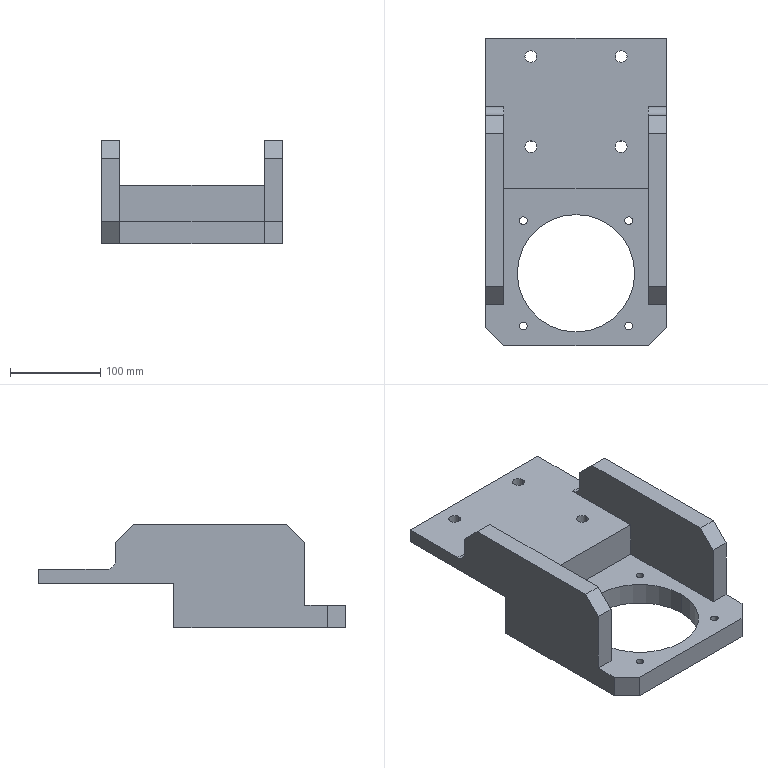Part | STEP file | LM-05-1159_default | 1 solid | 44 faces | box 200 x 340 x 115 mm | volume 1813258 mm3 | plane 24 | cylinder 20 | commonest cylinder face diameters 8.5 x8 13 x8 20 x2 130 x2